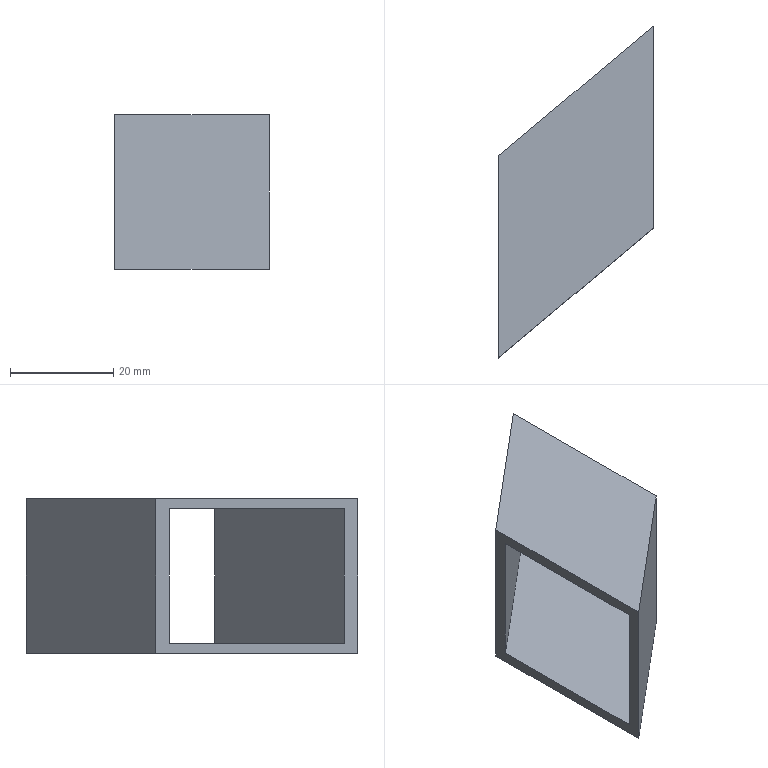Part | NX | features solid 2 | 1 solid | 10 faces | box 30 x 64.335 x 30 mm | volume 8772 mm3 | plane 10
STEP:
#1=CARTESIAN_POINT('',(0.,-85.173,-75.));
#2=VERTEX_POINT('',#1);
#3=CARTESIAN_POINT('',(0.,-124.335,-75.));
#4=VERTEX_POINT('',#3);
#5=CARTESIAN_POINT('',(0.,-188.558,-75.));
#6=DIRECTION('',(0.,-1.,0.));
#7=VECTOR('',#6,1000.);
#8=LINE('',#5,#7);
#9=EDGE_CURVE('',#2,#4,#8,.T.);
#10=ORIENTED_EDGE('',*,*,#9,.T.);
#11=CARTESIAN_POINT('',(0.,-124.335,-45.));
#12=VERTEX_POINT('',#11);
#13=CARTESIAN_POINT('',(0.,-124.335,-85.));
#14=DIRECTION('',(0.,0.,1.));
#15=VECTOR('',#14,1000.);
#16=LINE('',#13,#15);
#17=EDGE_CURVE('',#12,#4,#16,.F.);
#18=ORIENTED_EDGE('',*,*,#17,.F.);
#19=CARTESIAN_POINT('',(0.,-85.173,-45.));
#20=VERTEX_POINT('',#19);
#21=CARTESIAN_POINT('',(0.,115.,-45.));
#22=DIRECTION('',(0.,1.,0.));
#23=VECTOR('',#22,1000.);
#24=LINE('',#21,#23);
#25=EDGE_CURVE('',#20,#12,#24,.F.);
#26=ORIENTED_EDGE('',*,*,#25,.F.);
#27=CARTESIAN_POINT('',(0.,-85.173,-45.));
#28=DIRECTION('',(0.,0.,-1.));
#29=VECTOR('',#28,1000.);
#30=LINE('',#27,#29);
#31=EDGE_CURVE('',#20,#2,#30,.T.);
#32=ORIENTED_EDGE('',*,*,#31,.T.);
#33=EDGE_LOOP('',(#10,#18,#26,#32));
#34=FACE_BOUND('',#33,.T.);
#35=CARTESIAN_POINT('',(0.,-87.784,-73.));
#36=VERTEX_POINT('',#35);
#37=CARTESIAN_POINT('',(0.,-121.724,-73.));
#38=VERTEX_POINT('',#37);
#39=CARTESIAN_POINT('',(0.,115.,-73.));
#40=DIRECTION('',(0.,1.,0.));
#41=VECTOR('',#40,1000.);
#42=LINE('',#39,#41);
#43=EDGE_CURVE('',#36,#38,#42,.F.);
#44=ORIENTED_EDGE('',*,*,#43,.F.);
#45=CARTESIAN_POINT('',(0.,-87.784,-47.));
#46=VERTEX_POINT('',#45);
#47=CARTESIAN_POINT('',(0.,-87.784,-45.));
#48=DIRECTION('',(0.,0.,1.));
#49=VECTOR('',#48,1000.);
#50=LINE('',#47,#49);
#51=EDGE_CURVE('',#46,#36,#50,.F.);
#52=ORIENTED_EDGE('',*,*,#51,.F.);
#53=CARTESIAN_POINT('',(0.,-121.724,-47.));
#54=VERTEX_POINT('',#53);
#55=CARTESIAN_POINT('',(0.,115.,-47.));
#56=DIRECTION('',(0.,1.,0.));
#57=VECTOR('',#56,1000.);
#58=LINE('',#55,#57);
#59=EDGE_CURVE('',#46,#54,#58,.F.);
#60=ORIENTED_EDGE('',*,*,#59,.T.);
#61=CARTESIAN_POINT('',(0.,-121.724,-45.));
#62=DIRECTION('',(0.,0.,1.));
#63=VECTOR('',#62,1000.);
#64=LINE('',#61,#63);
#65=EDGE_CURVE('',#54,#38,#64,.F.);
#66=ORIENTED_EDGE('',*,*,#65,.T.);
#67=EDGE_LOOP('',(#44,#52,#60,#66));
#68=FACE_BOUND('',#67,.T.);
#69=CARTESIAN_POINT('',(0.,115.,-45.));
#70=DIRECTION('',(-1.,0.,0.));
#71=DIRECTION('',(0.,-1.,0.));
#72=AXIS2_PLACEMENT_3D('',#69,#70,#71);
#73=PLANE('',#72);
#74=ADVANCED_FACE('',(#34,#68),#73,.T.);
#75=CARTESIAN_POINT('',(30.,-60.,-75.));
#76=VERTEX_POINT('',#75);
#77=CARTESIAN_POINT('',(30.,-99.162,-75.));
#78=VERTEX_POINT('',#77);
#79=CARTESIAN_POINT('',(30.,-188.558,-75.));
#80=DIRECTION('',(0.,-1.,0.));
#81=VECTOR('',#80,1000.);
#82=LINE('',#79,#81);
#83=EDGE_CURVE('',#76,#78,#82,.T.);
#84=ORIENTED_EDGE('',*,*,#83,.F.);
#85=CARTESIAN_POINT('',(30.,-60.,-45.));
#86=VERTEX_POINT('',#85);
#87=CARTESIAN_POINT('',(30.,-60.,-45.));
#88=DIRECTION('',(0.,0.,-1.));
#89=VECTOR('',#88,1000.);
#90=LINE('',#87,#89);
#91=EDGE_CURVE('',#86,#76,#90,.T.);
#92=ORIENTED_EDGE('',*,*,#91,.F.);
#93=CARTESIAN_POINT('',(30.,-99.162,-45.));
#94=VERTEX_POINT('',#93);
#95=CARTESIAN_POINT('',(30.,115.,-45.));
#96=DIRECTION('',(0.,1.,0.));
#97=VECTOR('',#96,1000.);
#98=LINE('',#95,#97);
#99=EDGE_CURVE('',#86,#94,#98,.F.);
#100=ORIENTED_EDGE('',*,*,#99,.T.);
#101=CARTESIAN_POINT('',(30.,-99.162,-85.));
#102=DIRECTION('',(0.,0.,1.));
#103=VECTOR('',#102,1000.);
#104=LINE('',#101,#103);
#105=EDGE_CURVE('',#94,#78,#104,.F.);
#106=ORIENTED_EDGE('',*,*,#105,.T.);
#107=EDGE_LOOP('',(#84,#92,#100,#106));
#108=FACE_BOUND('',#107,.T.);
#109=CARTESIAN_POINT('',(30.,-62.611,-47.));
#110=VERTEX_POINT('',#109);
#111=CARTESIAN_POINT('',(30.,-62.611,-73.));
#112=VERTEX_POINT('',#111);
#113=CARTESIAN_POINT('',(30.,-62.611,-45.));
#114=DIRECTION('',(0.,0.,-1.));
#115=VECTOR('',#114,1000.);
#116=LINE('',#113,#115);
#117=EDGE_CURVE('',#110,#112,#116,.T.);
#118=ORIENTED_EDGE('',*,*,#117,.T.);
#119=CARTESIAN_POINT('',(30.,-96.551,-73.));
#120=VERTEX_POINT('',#119);
#121=CARTESIAN_POINT('',(30.,-188.558,-73.));
#122=DIRECTION('',(0.,-1.,0.));
#123=VECTOR('',#122,1000.);
#124=LINE('',#121,#123);
#125=EDGE_CURVE('',#112,#120,#124,.T.);
#126=ORIENTED_EDGE('',*,*,#125,.T.);
#127=CARTESIAN_POINT('',(30.,-96.551,-47.));
#128=VERTEX_POINT('',#127);
#129=CARTESIAN_POINT('',(30.,-96.551,-85.));
#130=DIRECTION('',(0.,0.,1.));
#131=VECTOR('',#130,1000.);
#132=LINE('',#129,#131);
#133=EDGE_CURVE('',#128,#120,#132,.F.);
#134=ORIENTED_EDGE('',*,*,#133,.F.);
#135=CARTESIAN_POINT('',(30.,115.,-47.));
#136=DIRECTION('',(0.,1.,0.));
#137=VECTOR('',#136,1000.);
#138=LINE('',#135,#137);
#139=EDGE_CURVE('',#110,#128,#138,.F.);
#140=ORIENTED_EDGE('',*,*,#139,.F.);
#141=EDGE_LOOP('',(#118,#126,#134,#140));
#142=FACE_BOUND('',#141,.T.);
#143=CARTESIAN_POINT('',(30.,115.,-45.));
#144=DIRECTION('',(-1.,0.,0.));
#145=DIRECTION('',(0.,-1.,0.));
#146=AXIS2_PLACEMENT_3D('',#143,#144,#145);
#147=PLANE('',#146);
#148=ADVANCED_FACE('',(#108,#142),#147,.F.);
#149=CARTESIAN_POINT('',(-123.209,-188.558,-75.));
#150=DIRECTION('',(-0.766,-0.6428,0.));
#151=VECTOR('',#150,1000.);
#152=LINE('',#149,#151);
#153=EDGE_CURVE('',#76,#2,#152,.T.);
#154=ORIENTED_EDGE('',*,*,#153,.T.);
#155=ORIENTED_EDGE('',*,*,#31,.F.);
#156=CARTESIAN_POINT('',(104.434,2.458,-45.));
#157=DIRECTION('',(0.766,0.6428,0.));
#158=VECTOR('',#157,1000.);
#159=LINE('',#156,#158);
#160=EDGE_CURVE('',#86,#20,#159,.F.);
#161=ORIENTED_EDGE('',*,*,#160,.F.);
#162=ORIENTED_EDGE('',*,*,#91,.T.);
#163=EDGE_LOOP('',(#154,#155,#161,#162));
#164=FACE_BOUND('',#163,.T.);
#165=CARTESIAN_POINT('',(-123.209,-188.558,-85.));
#166=DIRECTION('',(-0.6428,0.766,0.));
#167=DIRECTION('',(0.,0.,1.));
#168=AXIS2_PLACEMENT_3D('',#165,#166,#167);
#169=PLANE('',#168);
#170=ADVANCED_FACE('',(#164),#169,.T.);
#171=CARTESIAN_POINT('',(-103.925,-211.539,-75.));
#172=DIRECTION('',(-0.766,-0.6428,0.));
#173=VECTOR('',#172,1000.);
#174=LINE('',#171,#173);
#175=EDGE_CURVE('',#4,#78,#174,.F.);
#176=ORIENTED_EDGE('',*,*,#175,.T.);
#177=ORIENTED_EDGE('',*,*,#105,.F.);
#178=CARTESIAN_POINT('',(123.718,-20.524,-45.));
#179=DIRECTION('',(0.766,0.6428,0.));
#180=VECTOR('',#179,1000.);
#181=LINE('',#178,#180);
#182=EDGE_CURVE('',#12,#94,#181,.T.);
#183=ORIENTED_EDGE('',*,*,#182,.F.);
#184=ORIENTED_EDGE('',*,*,#17,.T.);
#185=EDGE_LOOP('',(#176,#177,#183,#184));
#186=FACE_BOUND('',#185,.T.);
#187=CARTESIAN_POINT('',(-103.925,-211.539,-85.));
#188=DIRECTION('',(-0.6428,0.766,0.));
#189=DIRECTION('',(0.,0.,1.));
#190=AXIS2_PLACEMENT_3D('',#187,#188,#189);
#191=PLANE('',#190);
#192=ADVANCED_FACE('',(#186),#191,.F.);
#193=ORIENTED_EDGE('',*,*,#99,.F.);
#194=ORIENTED_EDGE('',*,*,#160,.T.);
#195=ORIENTED_EDGE('',*,*,#25,.T.);
#196=ORIENTED_EDGE('',*,*,#182,.T.);
#197=EDGE_LOOP('',(#193,#194,#195,#196));
#198=FACE_BOUND('',#197,.T.);
#199=CARTESIAN_POINT('',(10.,115.,-45.));
#200=DIRECTION('',(0.,0.,-1.));
#201=DIRECTION('',(0.,-1.,0.));
#202=AXIS2_PLACEMENT_3D('',#199,#200,#201);
#203=PLANE('',#202);
#204=ADVANCED_FACE('',(#198),#203,.F.);
#205=ORIENTED_EDGE('',*,*,#83,.T.);
#206=ORIENTED_EDGE('',*,*,#175,.F.);
#207=ORIENTED_EDGE('',*,*,#9,.F.);
#208=ORIENTED_EDGE('',*,*,#153,.F.);
#209=EDGE_LOOP('',(#205,#206,#207,#208));
#210=FACE_BOUND('',#209,.T.);
#211=CARTESIAN_POINT('',(-123.209,-188.558,-75.));
#212=DIRECTION('',(0.,0.,1.));
#213=DIRECTION('',(0.6428,-0.766,0.));
#214=AXIS2_PLACEMENT_3D('',#211,#212,#213);
#215=PLANE('',#214);
#216=ADVANCED_FACE('',(#210),#215,.F.);
#217=CARTESIAN_POINT('',(105.72,0.9256,-47.));
#218=DIRECTION('',(0.766,0.6428,0.));
#219=VECTOR('',#218,1000.);
#220=LINE('',#217,#219);
#221=EDGE_CURVE('',#110,#46,#220,.F.);
#222=ORIENTED_EDGE('',*,*,#221,.T.);
#223=ORIENTED_EDGE('',*,*,#51,.T.);
#224=CARTESIAN_POINT('',(-121.923,-190.09,-73.));
#225=DIRECTION('',(-0.766,-0.6428,0.));
#226=VECTOR('',#225,1000.);
#227=LINE('',#224,#226);
#228=EDGE_CURVE('',#112,#36,#227,.T.);
#229=ORIENTED_EDGE('',*,*,#228,.F.);
#230=ORIENTED_EDGE('',*,*,#117,.F.);
#231=EDGE_LOOP('',(#222,#223,#229,#230));
#232=FACE_BOUND('',#231,.T.);
#233=CARTESIAN_POINT('',(-121.923,-190.09,-85.));
#234=DIRECTION('',(-0.6428,0.766,0.));
#235=DIRECTION('',(0.,0.,1.));
#236=AXIS2_PLACEMENT_3D('',#233,#234,#235);
#237=PLANE('',#236);
#238=ADVANCED_FACE('',(#232),#237,.F.);
#239=ORIENTED_EDGE('',*,*,#133,.T.);
#240=CARTESIAN_POINT('',(-105.211,-210.007,-73.));
#241=DIRECTION('',(-0.766,-0.6428,0.));
#242=VECTOR('',#241,1000.);
#243=LINE('',#240,#242);
#244=EDGE_CURVE('',#38,#120,#243,.F.);
#245=ORIENTED_EDGE('',*,*,#244,.F.);
#246=ORIENTED_EDGE('',*,*,#65,.F.);
#247=CARTESIAN_POINT('',(122.432,-18.992,-47.));
#248=DIRECTION('',(0.766,0.6428,0.));
#249=VECTOR('',#248,1000.);
#250=LINE('',#247,#249);
#251=EDGE_CURVE('',#54,#128,#250,.T.);
#252=ORIENTED_EDGE('',*,*,#251,.T.);
#253=EDGE_LOOP('',(#239,#245,#246,#252));
#254=FACE_BOUND('',#253,.T.);
#255=CARTESIAN_POINT('',(-105.211,-210.007,-85.));
#256=DIRECTION('',(-0.6428,0.766,0.));
#257=DIRECTION('',(0.,0.,1.));
#258=AXIS2_PLACEMENT_3D('',#255,#256,#257);
#259=PLANE('',#258);
#260=ADVANCED_FACE('',(#254),#259,.T.);
#261=ORIENTED_EDGE('',*,*,#139,.T.);
#262=ORIENTED_EDGE('',*,*,#251,.F.);
#263=ORIENTED_EDGE('',*,*,#59,.F.);
#264=ORIENTED_EDGE('',*,*,#221,.F.);
#265=EDGE_LOOP('',(#261,#262,#263,#264));
#266=FACE_BOUND('',#265,.T.);
#267=CARTESIAN_POINT('',(10.,115.,-47.));
#268=DIRECTION('',(0.,0.,-1.));
#269=DIRECTION('',(0.,-1.,0.));
#270=AXIS2_PLACEMENT_3D('',#267,#268,#269);
#271=PLANE('',#270);
#272=ADVANCED_FACE('',(#266),#271,.T.);
#273=ORIENTED_EDGE('',*,*,#228,.T.);
#274=ORIENTED_EDGE('',*,*,#43,.T.);
#275=ORIENTED_EDGE('',*,*,#244,.T.);
#276=ORIENTED_EDGE('',*,*,#125,.F.);
#277=EDGE_LOOP('',(#273,#274,#275,#276));
#278=FACE_BOUND('',#277,.T.);
#279=CARTESIAN_POINT('',(-123.209,-188.558,-73.));
#280=DIRECTION('',(0.,0.,1.));
#281=DIRECTION('',(0.6428,-0.766,0.));
#282=AXIS2_PLACEMENT_3D('',#279,#280,#281);
#283=PLANE('',#282);
#284=ADVANCED_FACE('',(#278),#283,.T.);
#285=CLOSED_SHELL('',(#74,#148,#170,#192,#204,#216,#238,#260,#272,#284));
#286=MANIFOLD_SOLID_BREP('',#285);
#287=(LENGTH_UNIT()NAMED_UNIT(*)SI_UNIT(.MILLI.,.METRE.));
#288=UNCERTAINTY_MEASURE_WITH_UNIT(LENGTH_MEASURE(0.00001),#287,'','');
#289=(NAMED_UNIT(*)PLANE_ANGLE_UNIT()SI_UNIT($,.RADIAN.));
#290=(NAMED_UNIT(*)SI_UNIT($,.STERADIAN.)SOLID_ANGLE_UNIT());
#291=(GEOMETRIC_REPRESENTATION_CONTEXT(3)GLOBAL_UNCERTAINTY_ASSIGNED_CONTEXT((#288))GLOBAL_UNIT_ASSIGNED_CONTEXT((#287,#289,#290))REPRESENTATION_CONTEXT('',''));
#292=ADVANCED_BREP_SHAPE_REPRESENTATION('',(#286),#291);